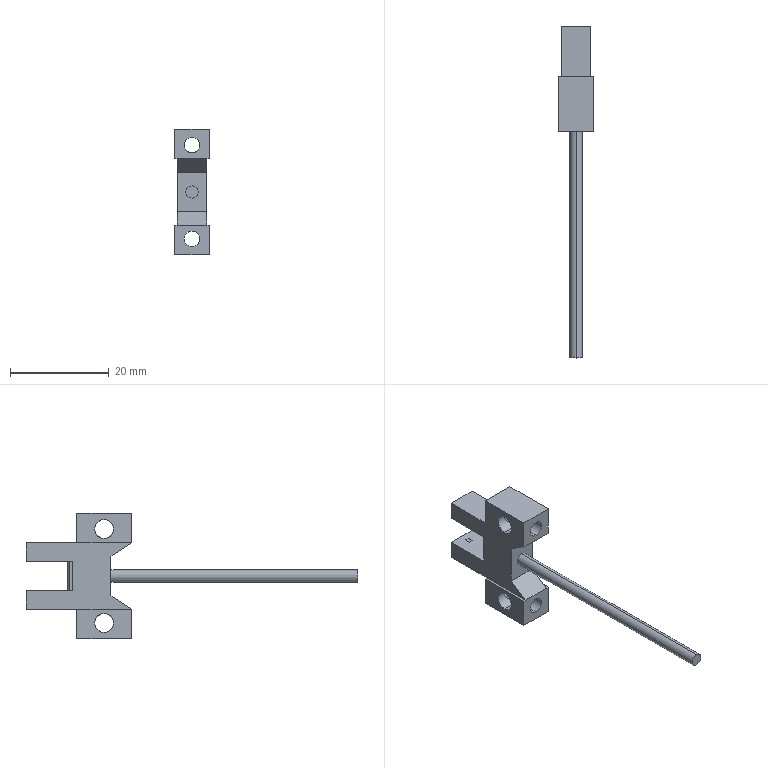Part | SolidWorks | features BaseBody 1 | 1 solid | 73 faces | box 7 x 67.2 x 25.4 mm | volume 2029 mm3 | plane 59 | cylinder 14 | commonest cylinder face diameters 3.2 x8 3.8 x4 2.5 x2